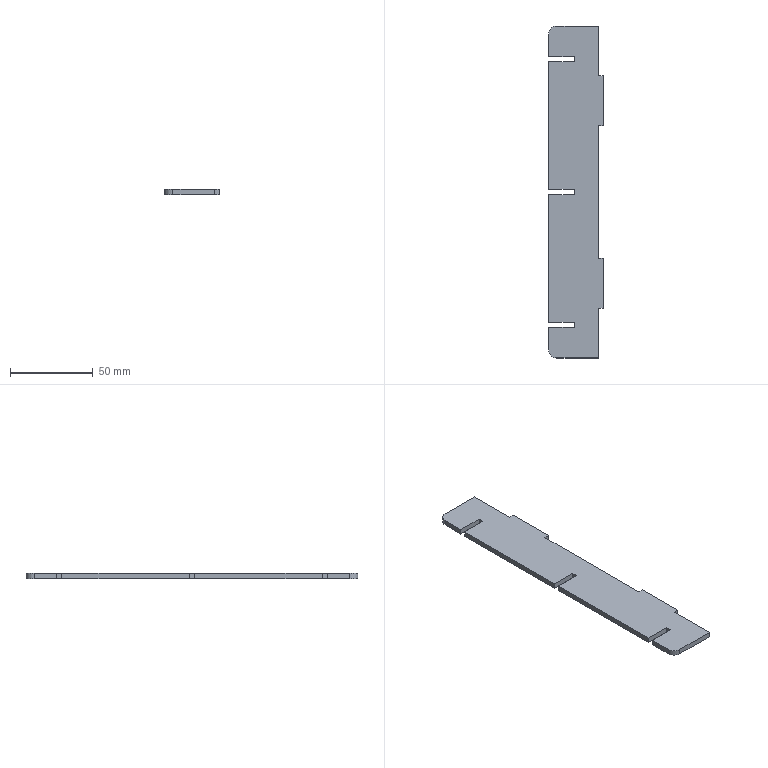Part | SolidWorks | features FlatPattern 1, SMBaseFlange 1, SheetMetal 1 | 1 solid | 28 faces | box 33 x 200 x 3.2 mm | volume 19266 mm3 | plane 26 | cylinder 2 | commonest cylinder face diameters 10 x2
STEP:
#1=CARTESIAN_POINT('',(108.501,81.943,0.));
#2=VERTEX_POINT('',#1);
#3=CARTESIAN_POINT('',(108.501,111.943,0.));
#4=VERTEX_POINT('',#3);
#5=CARTESIAN_POINT('',(108.501,111.943,0.));
#6=DIRECTION('',(0.,1.,0.));
#7=VECTOR('',#6,1000.);
#8=LINE('',#5,#7);
#9=EDGE_CURVE('',#2,#4,#8,.T.);
#10=ORIENTED_EDGE('',*,*,#9,.F.);
#11=CARTESIAN_POINT('',(108.501,81.943,-3.2));
#12=VERTEX_POINT('',#11);
#13=CARTESIAN_POINT('',(108.501,81.943,-3.2));
#14=DIRECTION('',(0.,0.,1.));
#15=VECTOR('',#14,1000.);
#16=LINE('',#13,#15);
#17=EDGE_CURVE('',#12,#2,#16,.T.);
#18=ORIENTED_EDGE('',*,*,#17,.F.);
#19=CARTESIAN_POINT('',(108.501,111.943,-3.2));
#20=VERTEX_POINT('',#19);
#21=CARTESIAN_POINT('',(108.501,111.943,-3.2));
#22=DIRECTION('',(0.,1.,0.));
#23=VECTOR('',#22,1000.);
#24=LINE('',#21,#23);
#25=EDGE_CURVE('',#12,#20,#24,.T.);
#26=ORIENTED_EDGE('',*,*,#25,.T.);
#27=CARTESIAN_POINT('',(108.501,111.943,-3.2));
#28=DIRECTION('',(0.,0.,1.));
#29=VECTOR('',#28,1000.);
#30=LINE('',#27,#29);
#31=EDGE_CURVE('',#20,#4,#30,.T.);
#32=ORIENTED_EDGE('',*,*,#31,.T.);
#33=EDGE_LOOP('',(#10,#18,#26,#32));
#34=FACE_OUTER_BOUND('',#33,.T.);
#35=CARTESIAN_POINT('',(108.501,111.943,-3.2));
#36=DIRECTION('',(1.,0.,0.));
#37=DIRECTION('',(0.,0.,-1.));
#38=AXIS2_PLACEMENT_3D('',#35,#36,#37);
#39=PLANE('',#38);
#40=ADVANCED_FACE('',(#34),#39,.T.);
#41=CARTESIAN_POINT('',(111.501,81.943,0.));
#42=VERTEX_POINT('',#41);
#43=CARTESIAN_POINT('',(108.501,81.943,0.));
#44=DIRECTION('',(-1.,0.,0.));
#45=VECTOR('',#44,1000.);
#46=LINE('',#43,#45);
#47=EDGE_CURVE('',#42,#2,#46,.T.);
#48=ORIENTED_EDGE('',*,*,#47,.F.);
#49=CARTESIAN_POINT('',(111.501,81.943,-3.2));
#50=VERTEX_POINT('',#49);
#51=CARTESIAN_POINT('',(111.501,81.943,-3.2));
#52=DIRECTION('',(0.,0.,1.));
#53=VECTOR('',#52,1000.);
#54=LINE('',#51,#53);
#55=EDGE_CURVE('',#50,#42,#54,.T.);
#56=ORIENTED_EDGE('',*,*,#55,.F.);
#57=CARTESIAN_POINT('',(108.501,81.943,-3.2));
#58=DIRECTION('',(-1.,0.,0.));
#59=VECTOR('',#58,1000.);
#60=LINE('',#57,#59);
#61=EDGE_CURVE('',#50,#12,#60,.T.);
#62=ORIENTED_EDGE('',*,*,#61,.T.);
#63=ORIENTED_EDGE('',*,*,#17,.T.);
#64=EDGE_LOOP('',(#48,#56,#62,#63));
#65=FACE_OUTER_BOUND('',#64,.T.);
#66=CARTESIAN_POINT('',(108.501,81.943,-3.2));
#67=DIRECTION('',(0.,1.,0.));
#68=DIRECTION('',(0.,0.,1.));
#69=AXIS2_PLACEMENT_3D('',#66,#67,#68);
#70=PLANE('',#69);
#71=ADVANCED_FACE('',(#65),#70,.T.);
#72=CARTESIAN_POINT('',(111.501,51.943,0.));
#73=VERTEX_POINT('',#72);
#74=CARTESIAN_POINT('',(111.501,81.943,0.));
#75=DIRECTION('',(0.,1.,0.));
#76=VECTOR('',#75,1000.);
#77=LINE('',#74,#76);
#78=EDGE_CURVE('',#73,#42,#77,.T.);
#79=ORIENTED_EDGE('',*,*,#78,.F.);
#80=CARTESIAN_POINT('',(111.501,51.943,-3.2));
#81=VERTEX_POINT('',#80);
#82=CARTESIAN_POINT('',(111.501,51.943,-3.2));
#83=DIRECTION('',(0.,0.,1.));
#84=VECTOR('',#83,1000.);
#85=LINE('',#82,#84);
#86=EDGE_CURVE('',#81,#73,#85,.T.);
#87=ORIENTED_EDGE('',*,*,#86,.F.);
#88=CARTESIAN_POINT('',(111.501,81.943,-3.2));
#89=DIRECTION('',(0.,1.,0.));
#90=VECTOR('',#89,1000.);
#91=LINE('',#88,#90);
#92=EDGE_CURVE('',#81,#50,#91,.T.);
#93=ORIENTED_EDGE('',*,*,#92,.T.);
#94=ORIENTED_EDGE('',*,*,#55,.T.);
#95=EDGE_LOOP('',(#79,#87,#93,#94));
#96=FACE_OUTER_BOUND('',#95,.T.);
#97=CARTESIAN_POINT('',(111.501,81.943,-3.2));
#98=DIRECTION('',(1.,0.,0.));
#99=DIRECTION('',(0.,1.,0.));
#100=AXIS2_PLACEMENT_3D('',#97,#98,#99);
#101=PLANE('',#100);
#102=ADVANCED_FACE('',(#96),#101,.T.);
#103=CARTESIAN_POINT('',(108.501,51.943,0.));
#104=VERTEX_POINT('',#103);
#105=CARTESIAN_POINT('',(111.501,51.943,0.));
#106=DIRECTION('',(1.,0.,0.));
#107=VECTOR('',#106,1000.);
#108=LINE('',#105,#107);
#109=EDGE_CURVE('',#104,#73,#108,.T.);
#110=ORIENTED_EDGE('',*,*,#109,.F.);
#111=CARTESIAN_POINT('',(108.501,51.943,-3.2));
#112=VERTEX_POINT('',#111);
#113=CARTESIAN_POINT('',(108.501,51.943,-3.2));
#114=DIRECTION('',(0.,0.,1.));
#115=VECTOR('',#114,1000.);
#116=LINE('',#113,#115);
#117=EDGE_CURVE('',#112,#104,#116,.T.);
#118=ORIENTED_EDGE('',*,*,#117,.F.);
#119=CARTESIAN_POINT('',(111.501,51.943,-3.2));
#120=DIRECTION('',(1.,0.,0.));
#121=VECTOR('',#120,1000.);
#122=LINE('',#119,#121);
#123=EDGE_CURVE('',#112,#81,#122,.T.);
#124=ORIENTED_EDGE('',*,*,#123,.T.);
#125=ORIENTED_EDGE('',*,*,#86,.T.);
#126=EDGE_LOOP('',(#110,#118,#124,#125));
#127=FACE_OUTER_BOUND('',#126,.T.);
#128=CARTESIAN_POINT('',(111.501,51.943,-3.2));
#129=DIRECTION('',(0.,-1.,0.));
#130=DIRECTION('',(0.,0.,-1.));
#131=AXIS2_PLACEMENT_3D('',#128,#129,#130);
#132=PLANE('',#131);
#133=ADVANCED_FACE('',(#127),#132,.T.);
#134=CARTESIAN_POINT('',(108.501,-28.057,0.));
#135=VERTEX_POINT('',#134);
#136=CARTESIAN_POINT('',(108.501,51.943,0.));
#137=DIRECTION('',(0.,1.,0.));
#138=VECTOR('',#137,1000.);
#139=LINE('',#136,#138);
#140=EDGE_CURVE('',#135,#104,#139,.T.);
#141=ORIENTED_EDGE('',*,*,#140,.F.);
#142=CARTESIAN_POINT('',(108.501,-28.057,-3.2));
#143=VERTEX_POINT('',#142);
#144=CARTESIAN_POINT('',(108.501,-28.057,-3.2));
#145=DIRECTION('',(0.,0.,1.));
#146=VECTOR('',#145,1000.);
#147=LINE('',#144,#146);
#148=EDGE_CURVE('',#143,#135,#147,.T.);
#149=ORIENTED_EDGE('',*,*,#148,.F.);
#150=CARTESIAN_POINT('',(108.501,51.943,-3.2));
#151=DIRECTION('',(0.,1.,0.));
#152=VECTOR('',#151,1000.);
#153=LINE('',#150,#152);
#154=EDGE_CURVE('',#143,#112,#153,.T.);
#155=ORIENTED_EDGE('',*,*,#154,.T.);
#156=ORIENTED_EDGE('',*,*,#117,.T.);
#157=EDGE_LOOP('',(#141,#149,#155,#156));
#158=FACE_OUTER_BOUND('',#157,.T.);
#159=CARTESIAN_POINT('',(108.501,51.943,-3.2));
#160=DIRECTION('',(1.,0.,0.));
#161=DIRECTION('',(0.,0.,-1.));
#162=AXIS2_PLACEMENT_3D('',#159,#160,#161);
#163=PLANE('',#162);
#164=ADVANCED_FACE('',(#158),#163,.T.);
#165=CARTESIAN_POINT('',(111.501,-28.057,0.));
#166=VERTEX_POINT('',#165);
#167=CARTESIAN_POINT('',(111.501,-28.057,0.));
#168=DIRECTION('',(-1.,0.,0.));
#169=VECTOR('',#168,1000.);
#170=LINE('',#167,#169);
#171=EDGE_CURVE('',#166,#135,#170,.T.);
#172=ORIENTED_EDGE('',*,*,#171,.F.);
#173=CARTESIAN_POINT('',(111.501,-28.057,-3.2));
#174=VERTEX_POINT('',#173);
#175=CARTESIAN_POINT('',(111.501,-28.057,-3.2));
#176=DIRECTION('',(0.,0.,1.));
#177=VECTOR('',#176,1000.);
#178=LINE('',#175,#177);
#179=EDGE_CURVE('',#174,#166,#178,.T.);
#180=ORIENTED_EDGE('',*,*,#179,.F.);
#181=CARTESIAN_POINT('',(111.501,-28.057,-3.2));
#182=DIRECTION('',(-1.,0.,0.));
#183=VECTOR('',#182,1000.);
#184=LINE('',#181,#183);
#185=EDGE_CURVE('',#174,#143,#184,.T.);
#186=ORIENTED_EDGE('',*,*,#185,.T.);
#187=ORIENTED_EDGE('',*,*,#148,.T.);
#188=EDGE_LOOP('',(#172,#180,#186,#187));
#189=FACE_OUTER_BOUND('',#188,.T.);
#190=CARTESIAN_POINT('',(111.501,-28.057,-3.2));
#191=DIRECTION('',(0.,1.,0.));
#192=DIRECTION('',(0.,0.,1.));
#193=AXIS2_PLACEMENT_3D('',#190,#191,#192);
#194=PLANE('',#193);
#195=ADVANCED_FACE('',(#189),#194,.T.);
#196=CARTESIAN_POINT('',(111.501,-58.057,0.));
#197=VERTEX_POINT('',#196);
#198=CARTESIAN_POINT('',(111.501,-58.057,0.));
#199=DIRECTION('',(0.,1.,0.));
#200=VECTOR('',#199,1000.);
#201=LINE('',#198,#200);
#202=EDGE_CURVE('',#197,#166,#201,.T.);
#203=ORIENTED_EDGE('',*,*,#202,.F.);
#204=CARTESIAN_POINT('',(111.501,-58.057,-3.2));
#205=VERTEX_POINT('',#204);
#206=CARTESIAN_POINT('',(111.501,-58.057,-3.2));
#207=DIRECTION('',(0.,0.,1.));
#208=VECTOR('',#207,1000.);
#209=LINE('',#206,#208);
#210=EDGE_CURVE('',#205,#197,#209,.T.);
#211=ORIENTED_EDGE('',*,*,#210,.F.);
#212=CARTESIAN_POINT('',(111.501,-58.057,-3.2));
#213=DIRECTION('',(0.,1.,0.));
#214=VECTOR('',#213,1000.);
#215=LINE('',#212,#214);
#216=EDGE_CURVE('',#205,#174,#215,.T.);
#217=ORIENTED_EDGE('',*,*,#216,.T.);
#218=ORIENTED_EDGE('',*,*,#179,.T.);
#219=EDGE_LOOP('',(#203,#211,#217,#218));
#220=FACE_OUTER_BOUND('',#219,.T.);
#221=CARTESIAN_POINT('',(111.501,-58.057,-3.2));
#222=DIRECTION('',(1.,0.,0.));
#223=DIRECTION('',(0.,0.,-1.));
#224=AXIS2_PLACEMENT_3D('',#221,#222,#223);
#225=PLANE('',#224);
#226=ADVANCED_FACE('',(#220),#225,.T.);
#227=CARTESIAN_POINT('',(108.501,-58.057,0.));
#228=VERTEX_POINT('',#227);
#229=CARTESIAN_POINT('',(108.501,-58.057,0.));
#230=DIRECTION('',(1.,0.,0.));
#231=VECTOR('',#230,1000.);
#232=LINE('',#229,#231);
#233=EDGE_CURVE('',#228,#197,#232,.T.);
#234=ORIENTED_EDGE('',*,*,#233,.F.);
#235=CARTESIAN_POINT('',(108.501,-58.057,-3.2));
#236=VERTEX_POINT('',#235);
#237=CARTESIAN_POINT('',(108.501,-58.057,-3.2));
#238=DIRECTION('',(0.,0.,1.));
#239=VECTOR('',#238,1000.);
#240=LINE('',#237,#239);
#241=EDGE_CURVE('',#236,#228,#240,.T.);
#242=ORIENTED_EDGE('',*,*,#241,.F.);
#243=CARTESIAN_POINT('',(108.501,-58.057,-3.2));
#244=DIRECTION('',(1.,0.,0.));
#245=VECTOR('',#244,1000.);
#246=LINE('',#243,#245);
#247=EDGE_CURVE('',#236,#205,#246,.T.);
#248=ORIENTED_EDGE('',*,*,#247,.T.);
#249=ORIENTED_EDGE('',*,*,#210,.T.);
#250=EDGE_LOOP('',(#234,#242,#248,#249));
#251=FACE_OUTER_BOUND('',#250,.T.);
#252=CARTESIAN_POINT('',(108.501,-58.057,-3.2));
#253=DIRECTION('',(0.,-1.,0.));
#254=DIRECTION('',(0.,0.,-1.));
#255=AXIS2_PLACEMENT_3D('',#252,#253,#254);
#256=PLANE('',#255);
#257=ADVANCED_FACE('',(#251),#256,.T.);
#258=CARTESIAN_POINT('',(108.501,-88.057,0.));
#259=VERTEX_POINT('',#258);
#260=CARTESIAN_POINT('',(108.501,-58.057,0.));
#261=DIRECTION('',(0.,1.,0.));
#262=VECTOR('',#261,1000.);
#263=LINE('',#260,#262);
#264=EDGE_CURVE('',#259,#228,#263,.T.);
#265=ORIENTED_EDGE('',*,*,#264,.F.);
#266=CARTESIAN_POINT('',(108.501,-88.057,-3.2));
#267=VERTEX_POINT('',#266);
#268=CARTESIAN_POINT('',(108.501,-88.057,-3.2));
#269=DIRECTION('',(0.,0.,1.));
#270=VECTOR('',#269,1000.);
#271=LINE('',#268,#270);
#272=EDGE_CURVE('',#267,#259,#271,.T.);
#273=ORIENTED_EDGE('',*,*,#272,.F.);
#274=CARTESIAN_POINT('',(108.501,-58.057,-3.2));
#275=DIRECTION('',(0.,1.,0.));
#276=VECTOR('',#275,1000.);
#277=LINE('',#274,#276);
#278=EDGE_CURVE('',#267,#236,#277,.T.);
#279=ORIENTED_EDGE('',*,*,#278,.T.);
#280=ORIENTED_EDGE('',*,*,#241,.T.);
#281=EDGE_LOOP('',(#265,#273,#279,#280));
#282=FACE_OUTER_BOUND('',#281,.T.);
#283=CARTESIAN_POINT('',(108.501,-58.057,-3.2));
#284=DIRECTION('',(1.,0.,0.));
#285=DIRECTION('',(0.,1.,0.));
#286=AXIS2_PLACEMENT_3D('',#283,#284,#285);
#287=PLANE('',#286);
#288=ADVANCED_FACE('',(#282),#287,.T.);
#289=CARTESIAN_POINT('',(83.501,-88.057,0.));
#290=VERTEX_POINT('',#289);
#291=CARTESIAN_POINT('',(108.501,-88.057,0.));
#292=DIRECTION('',(1.,0.,0.));
#293=VECTOR('',#292,1000.);
#294=LINE('',#291,#293);
#295=EDGE_CURVE('',#290,#259,#294,.T.);
#296=ORIENTED_EDGE('',*,*,#295,.F.);
#297=CARTESIAN_POINT('',(83.501,-88.057,-3.2));
#298=VERTEX_POINT('',#297);
#299=CARTESIAN_POINT('',(83.501,-88.057,-3.2));
#300=DIRECTION('',(0.,0.,1.));
#301=VECTOR('',#300,1000.);
#302=LINE('',#299,#301);
#303=EDGE_CURVE('',#298,#290,#302,.T.);
#304=ORIENTED_EDGE('',*,*,#303,.F.);
#305=CARTESIAN_POINT('',(108.501,-88.057,-3.2));
#306=DIRECTION('',(1.,0.,0.));
#307=VECTOR('',#306,1000.);
#308=LINE('',#305,#307);
#309=EDGE_CURVE('',#298,#267,#308,.T.);
#310=ORIENTED_EDGE('',*,*,#309,.T.);
#311=ORIENTED_EDGE('',*,*,#272,.T.);
#312=EDGE_LOOP('',(#296,#304,#310,#311));
#313=FACE_OUTER_BOUND('',#312,.T.);
#314=CARTESIAN_POINT('',(108.501,-88.057,-3.2));
#315=DIRECTION('',(0.,-1.,0.));
#316=DIRECTION('',(0.,0.,-1.));
#317=AXIS2_PLACEMENT_3D('',#314,#315,#316);
#318=PLANE('',#317);
#319=ADVANCED_FACE('',(#313),#318,.T.);
#320=CARTESIAN_POINT('',(78.501,-83.057,0.));
#321=VERTEX_POINT('',#320);
#322=CARTESIAN_POINT('',(83.501,-83.057,0.));
#323=DIRECTION('',(0.,0.,1.));
#324=DIRECTION('',(-1.,0.,0.));
#325=AXIS2_PLACEMENT_3D('',#322,#323,#324);
#326=CIRCLE('',#325,5.);
#327=EDGE_CURVE('',#321,#290,#326,.T.);
#328=ORIENTED_EDGE('',*,*,#327,.F.);
#329=CARTESIAN_POINT('',(78.501,-83.057,-3.2));
#330=VERTEX_POINT('',#329);
#331=CARTESIAN_POINT('',(78.501,-83.057,-3.2));
#332=DIRECTION('',(0.,0.,1.));
#333=VECTOR('',#332,1000.);
#334=LINE('',#331,#333);
#335=EDGE_CURVE('',#330,#321,#334,.T.);
#336=ORIENTED_EDGE('',*,*,#335,.F.);
#337=CARTESIAN_POINT('',(83.501,-83.057,-3.2));
#338=DIRECTION('',(0.,0.,1.));
#339=DIRECTION('',(-1.,0.,0.));
#340=AXIS2_PLACEMENT_3D('',#337,#338,#339);
#341=CIRCLE('',#340,5.);
#342=EDGE_CURVE('',#330,#298,#341,.T.);
#343=ORIENTED_EDGE('',*,*,#342,.T.);
#344=ORIENTED_EDGE('',*,*,#303,.T.);
#345=EDGE_LOOP('',(#328,#336,#343,#344));
#346=FACE_OUTER_BOUND('',#345,.T.);
#347=CARTESIAN_POINT('',(83.501,-83.057,-3.2));
#348=DIRECTION('',(0.,0.,1.));
#349=DIRECTION('',(1.,0.,0.));
#350=AXIS2_PLACEMENT_3D('',#347,#348,#349);
#351=CYLINDRICAL_SURFACE('',#350,5.);
#352=ADVANCED_FACE('',(#346),#351,.T.);
#353=CARTESIAN_POINT('',(78.501,-69.657,0.));
#354=VERTEX_POINT('',#353);
#355=CARTESIAN_POINT('',(78.501,-69.657,0.));
#356=DIRECTION('',(0.,-1.,0.));
#357=VECTOR('',#356,1000.);
#358=LINE('',#355,#357);
#359=EDGE_CURVE('',#354,#321,#358,.T.);
#360=ORIENTED_EDGE('',*,*,#359,.F.);
#361=CARTESIAN_POINT('',(78.501,-69.657,-3.2));
#362=VERTEX_POINT('',#361);
#363=CARTESIAN_POINT('',(78.501,-69.657,-3.2));
#364=DIRECTION('',(0.,0.,1.));
#365=VECTOR('',#364,1000.);
#366=LINE('',#363,#365);
#367=EDGE_CURVE('',#362,#354,#366,.T.);
#368=ORIENTED_EDGE('',*,*,#367,.F.);
#369=CARTESIAN_POINT('',(78.501,-69.657,-3.2));
#370=DIRECTION('',(0.,-1.,0.));
#371=VECTOR('',#370,1000.);
#372=LINE('',#369,#371);
#373=EDGE_CURVE('',#362,#330,#372,.T.);
#374=ORIENTED_EDGE('',*,*,#373,.T.);
#375=ORIENTED_EDGE('',*,*,#335,.T.);
#376=EDGE_LOOP('',(#360,#368,#374,#375));
#377=FACE_OUTER_BOUND('',#376,.T.);
#378=CARTESIAN_POINT('',(78.501,-69.657,-3.2));
#379=DIRECTION('',(-1.,0.,0.));
#380=DIRECTION('',(0.,0.,1.));
#381=AXIS2_PLACEMENT_3D('',#378,#379,#380);
#382=PLANE('',#381);
#383=ADVANCED_FACE('',(#377),#382,.T.);
#384=CARTESIAN_POINT('',(94.001,-69.657,0.));
#385=VERTEX_POINT('',#384);
#386=CARTESIAN_POINT('',(94.001,-69.657,0.));
#387=DIRECTION('',(-1.,0.,0.));
#388=VECTOR('',#387,1000.);
#389=LINE('',#386,#388);
#390=EDGE_CURVE('',#385,#354,#389,.T.);
#391=ORIENTED_EDGE('',*,*,#390,.F.);
#392=CARTESIAN_POINT('',(94.001,-69.657,-3.2));
#393=VERTEX_POINT('',#392);
#394=CARTESIAN_POINT('',(94.001,-69.657,-3.2));
#395=DIRECTION('',(0.,0.,1.));
#396=VECTOR('',#395,1000.);
#397=LINE('',#394,#396);
#398=EDGE_CURVE('',#393,#385,#397,.T.);
#399=ORIENTED_EDGE('',*,*,#398,.F.);
#400=CARTESIAN_POINT('',(94.001,-69.657,-3.2));
#401=DIRECTION('',(-1.,0.,0.));
#402=VECTOR('',#401,1000.);
#403=LINE('',#400,#402);
#404=EDGE_CURVE('',#393,#362,#403,.T.);
#405=ORIENTED_EDGE('',*,*,#404,.T.);
#406=ORIENTED_EDGE('',*,*,#367,.T.);
#407=EDGE_LOOP('',(#391,#399,#405,#406));
#408=FACE_OUTER_BOUND('',#407,.T.);
#409=CARTESIAN_POINT('',(94.001,-69.657,-3.2));
#410=DIRECTION('',(0.,1.,0.));
#411=DIRECTION('',(0.,0.,1.));
#412=AXIS2_PLACEMENT_3D('',#409,#410,#411);
#413=PLANE('',#412);
#414=ADVANCED_FACE('',(#408),#413,.T.);
#415=CARTESIAN_POINT('',(94.001,-66.457,0.));
#416=VERTEX_POINT('',#415);
#417=CARTESIAN_POINT('',(94.001,-66.457,0.));
#418=DIRECTION('',(0.,-1.,0.));
#419=VECTOR('',#418,1000.);
#420=LINE('',#417,#419);
#421=EDGE_CURVE('',#416,#385,#420,.T.);
#422=ORIENTED_EDGE('',*,*,#421,.F.);
#423=CARTESIAN_POINT('',(94.001,-66.457,-3.2));
#424=VERTEX_POINT('',#423);
#425=CARTESIAN_POINT('',(94.001,-66.457,-3.2));
#426=DIRECTION('',(0.,0.,1.));
#427=VECTOR('',#426,1000.);
#428=LINE('',#425,#427);
#429=EDGE_CURVE('',#424,#416,#428,.T.);
#430=ORIENTED_EDGE('',*,*,#429,.F.);
#431=CARTESIAN_POINT('',(94.001,-66.457,-3.2));
#432=DIRECTION('',(0.,-1.,0.));
#433=VECTOR('',#432,1000.);
#434=LINE('',#431,#433);
#435=EDGE_CURVE('',#424,#393,#434,.T.);
#436=ORIENTED_EDGE('',*,*,#435,.T.);
#437=ORIENTED_EDGE('',*,*,#398,.T.);
#438=EDGE_LOOP('',(#422,#430,#436,#437));
#439=FACE_OUTER_BOUND('',#438,.T.);
#440=CARTESIAN_POINT('',(94.001,-66.457,-3.2));
#441=DIRECTION('',(-1.,0.,0.));
#442=DIRECTION('',(0.,0.,1.));
#443=AXIS2_PLACEMENT_3D('',#440,#441,#442);
#444=PLANE('',#443);
#445=ADVANCED_FACE('',(#439),#444,.T.);
#446=CARTESIAN_POINT('',(78.501,-66.457,0.));
#447=VERTEX_POINT('',#446);
#448=CARTESIAN_POINT('',(78.501,-66.457,0.));
#449=DIRECTION('',(1.,0.,0.));
#450=VECTOR('',#449,1000.);
#451=LINE('',#448,#450);
#452=EDGE_CURVE('',#447,#416,#451,.T.);
#453=ORIENTED_EDGE('',*,*,#452,.F.);
#454=CARTESIAN_POINT('',(78.501,-66.457,-3.2));
#455=VERTEX_POINT('',#454);
#456=CARTESIAN_POINT('',(78.501,-66.457,-3.2));
#457=DIRECTION('',(0.,0.,1.));
#458=VECTOR('',#457,1000.);
#459=LINE('',#456,#458);
#460=EDGE_CURVE('',#455,#447,#459,.T.);
#461=ORIENTED_EDGE('',*,*,#460,.F.);
#462=CARTESIAN_POINT('',(78.501,-66.457,-3.2));
#463=DIRECTION('',(1.,0.,0.));
#464=VECTOR('',#463,1000.);
#465=LINE('',#462,#464);
#466=EDGE_CURVE('',#455,#424,#465,.T.);
#467=ORIENTED_EDGE('',*,*,#466,.T.);
#468=ORIENTED_EDGE('',*,*,#429,.T.);
#469=EDGE_LOOP('',(#453,#461,#467,#468));
#470=FACE_OUTER_BOUND('',#469,.T.);
#471=CARTESIAN_POINT('',(78.501,-66.457,-3.2));
#472=DIRECTION('',(0.,-1.,0.));
#473=DIRECTION('',(0.,0.,-1.));
#474=AXIS2_PLACEMENT_3D('',#471,#472,#473);
#475=PLANE('',#474);
#476=ADVANCED_FACE('',(#470),#475,.T.);
#477=CARTESIAN_POINT('',(78.501,10.343,0.));
#478=VERTEX_POINT('',#477);
#479=CARTESIAN_POINT('',(78.501,10.343,0.));
#480=DIRECTION('',(0.,-1.,0.));
#481=VECTOR('',#480,1000.);
#482=LINE('',#479,#481);
#483=EDGE_CURVE('',#478,#447,#482,.T.);
#484=ORIENTED_EDGE('',*,*,#483,.F.);
#485=CARTESIAN_POINT('',(78.501,10.343,-3.2));
#486=VERTEX_POINT('',#485);
#487=CARTESIAN_POINT('',(78.501,10.343,-3.2));
#488=DIRECTION('',(0.,0.,1.));
#489=VECTOR('',#488,1000.);
#490=LINE('',#487,#489);
#491=EDGE_CURVE('',#486,#478,#490,.T.);
#492=ORIENTED_EDGE('',*,*,#491,.F.);
#493=CARTESIAN_POINT('',(78.501,10.343,-3.2));
#494=DIRECTION('',(0.,-1.,0.));
#495=VECTOR('',#494,1000.);
#496=LINE('',#493,#495);
#497=EDGE_CURVE('',#486,#455,#496,.T.);
#498=ORIENTED_EDGE('',*,*,#497,.T.);
#499=ORIENTED_EDGE('',*,*,#460,.T.);
#500=EDGE_LOOP('',(#484,#492,#498,#499));
#501=FACE_OUTER_BOUND('',#500,.T.);
#502=CARTESIAN_POINT('',(78.501,10.343,-3.2));
#503=DIRECTION('',(-1.,0.,0.));
#504=DIRECTION('',(0.,0.,1.));
#505=AXIS2_PLACEMENT_3D('',#502,#503,#504);
#506=PLANE('',#505);
#507=ADVANCED_FACE('',(#501),#506,.T.);
#508=CARTESIAN_POINT('',(94.001,10.343,0.));
#509=VERTEX_POINT('',#508);
#510=CARTESIAN_POINT('',(94.001,10.343,0.));
#511=DIRECTION('',(-1.,0.,0.));
#512=VECTOR('',#511,1000.);
#513=LINE('',#510,#512);
#514=EDGE_CURVE('',#509,#478,#513,.T.);
#515=ORIENTED_EDGE('',*,*,#514,.F.);
#516=CARTESIAN_POINT('',(94.001,10.343,-3.2));
#517=VERTEX_POINT('',#516);
#518=CARTESIAN_POINT('',(94.001,10.343,-3.2));
#519=DIRECTION('',(0.,0.,1.));
#520=VECTOR('',#519,1000.);
#521=LINE('',#518,#520);
#522=EDGE_CURVE('',#517,#509,#521,.T.);
#523=ORIENTED_EDGE('',*,*,#522,.F.);
#524=CARTESIAN_POINT('',(94.001,10.343,-3.2));
#525=DIRECTION('',(-1.,0.,0.));
#526=VECTOR('',#525,1000.);
#527=LINE('',#524,#526);
#528=EDGE_CURVE('',#517,#486,#527,.T.);
#529=ORIENTED_EDGE('',*,*,#528,.T.);
#530=ORIENTED_EDGE('',*,*,#491,.T.);
#531=EDGE_LOOP('',(#515,#523,#529,#530));
#532=FACE_OUTER_BOUND('',#531,.T.);
#533=CARTESIAN_POINT('',(94.001,10.343,-3.2));
#534=DIRECTION('',(0.,1.,0.));
#535=DIRECTION('',(-1.,0.,0.));
#536=AXIS2_PLACEMENT_3D('',#533,#534,#535);
#537=PLANE('',#536);
#538=ADVANCED_FACE('',(#532),#537,.T.);
#539=CARTESIAN_POINT('',(94.001,13.543,0.));
#540=VERTEX_POINT('',#539);
#541=CARTESIAN_POINT('',(94.001,13.543,0.));
#542=DIRECTION('',(0.,-1.,0.));
#543=VECTOR('',#542,1000.);
#544=LINE('',#541,#543);
#545=EDGE_CURVE('',#540,#509,#544,.T.);
#546=ORIENTED_EDGE('',*,*,#545,.F.);
#547=CARTESIAN_POINT('',(94.001,13.543,-3.2));
#548=VERTEX_POINT('',#547);
#549=CARTESIAN_POINT('',(94.001,13.543,-3.2));
#550=DIRECTION('',(0.,0.,1.));
#551=VECTOR('',#550,1000.);
#552=LINE('',#549,#551);
#553=EDGE_CURVE('',#548,#540,#552,.T.);
#554=ORIENTED_EDGE('',*,*,#553,.F.);
#555=CARTESIAN_POINT('',(94.001,13.543,-3.2));
#556=DIRECTION('',(0.,-1.,0.));
#557=VECTOR('',#556,1000.);
#558=LINE('',#555,#557);
#559=EDGE_CURVE('',#548,#517,#558,.T.);
#560=ORIENTED_EDGE('',*,*,#559,.T.);
#561=ORIENTED_EDGE('',*,*,#522,.T.);
#562=EDGE_LOOP('',(#546,#554,#560,#561));
#563=FACE_OUTER_BOUND('',#562,.T.);
#564=CARTESIAN_POINT('',(94.001,13.543,-3.2));
#565=DIRECTION('',(-1.,0.,0.));
#566=DIRECTION('',(0.,-1.,0.));
#567=AXIS2_PLACEMENT_3D('',#564,#565,#566);
#568=PLANE('',#567);
#569=ADVANCED_FACE('',(#563),#568,.T.);
#570=CARTESIAN_POINT('',(78.501,13.543,0.));
#571=VERTEX_POINT('',#570);
#572=CARTESIAN_POINT('',(78.501,13.543,0.));
#573=DIRECTION('',(1.,0.,0.));
#574=VECTOR('',#573,1000.);
#575=LINE('',#572,#574);
#576=EDGE_CURVE('',#571,#540,#575,.T.);
#577=ORIENTED_EDGE('',*,*,#576,.F.);
#578=CARTESIAN_POINT('',(78.501,13.543,-3.2));
#579=VERTEX_POINT('',#578);
#580=CARTESIAN_POINT('',(78.501,13.543,-3.2));
#581=DIRECTION('',(0.,0.,1.));
#582=VECTOR('',#581,1000.);
#583=LINE('',#580,#582);
#584=EDGE_CURVE('',#579,#571,#583,.T.);
#585=ORIENTED_EDGE('',*,*,#584,.F.);
#586=CARTESIAN_POINT('',(78.501,13.543,-3.2));
#587=DIRECTION('',(1.,0.,0.));
#588=VECTOR('',#587,1000.);
#589=LINE('',#586,#588);
#590=EDGE_CURVE('',#579,#548,#589,.T.);
#591=ORIENTED_EDGE('',*,*,#590,.T.);
#592=ORIENTED_EDGE('',*,*,#553,.T.);
#593=EDGE_LOOP('',(#577,#585,#591,#592));
#594=FACE_OUTER_BOUND('',#593,.T.);
#595=CARTESIAN_POINT('',(78.501,13.543,-3.2));
#596=DIRECTION('',(0.,-1.,0.));
#597=DIRECTION('',(1.,0.,0.));
#598=AXIS2_PLACEMENT_3D('',#595,#596,#597);
#599=PLANE('',#598);
#600=ADVANCED_FACE('',(#594),#599,.T.);
#601=CARTESIAN_POINT('',(78.501,90.343,0.));
#602=VERTEX_POINT('',#601);
#603=CARTESIAN_POINT('',(78.501,90.343,0.));
#604=DIRECTION('',(0.,-1.,0.));
#605=VECTOR('',#604,1000.);
#606=LINE('',#603,#605);
#607=EDGE_CURVE('',#602,#571,#606,.T.);
#608=ORIENTED_EDGE('',*,*,#607,.F.);
#609=CARTESIAN_POINT('',(78.501,90.343,-3.2));
#610=VERTEX_POINT('',#609);
#611=CARTESIAN_POINT('',(78.501,90.343,-3.2));
#612=DIRECTION('',(0.,0.,1.));
#613=VECTOR('',#612,1000.);
#614=LINE('',#611,#613);
#615=EDGE_CURVE('',#610,#602,#614,.T.);
#616=ORIENTED_EDGE('',*,*,#615,.F.);
#617=CARTESIAN_POINT('',(78.501,90.343,-3.2));
#618=DIRECTION('',(0.,-1.,0.));
#619=VECTOR('',#618,1000.);
#620=LINE('',#617,#619);
#621=EDGE_CURVE('',#610,#579,#620,.T.);
#622=ORIENTED_EDGE('',*,*,#621,.T.);
#623=ORIENTED_EDGE('',*,*,#584,.T.);
#624=EDGE_LOOP('',(#608,#616,#622,#623));
#625=FACE_OUTER_BOUND('',#624,.T.);
#626=CARTESIAN_POINT('',(78.501,90.343,-3.2));
#627=DIRECTION('',(-1.,0.,0.));
#628=DIRECTION('',(0.,-1.,0.));
#629=AXIS2_PLACEMENT_3D('',#626,#627,#628);
#630=PLANE('',#629);
#631=ADVANCED_FACE('',(#625),#630,.T.);
#632=CARTESIAN_POINT('',(94.001,90.343,0.));
#633=VERTEX_POINT('',#632);
#634=CARTESIAN_POINT('',(94.001,90.343,0.));
#635=DIRECTION('',(-1.,0.,0.));
#636=VECTOR('',#635,1000.);
#637=LINE('',#634,#636);
#638=EDGE_CURVE('',#633,#602,#637,.T.);
#639=ORIENTED_EDGE('',*,*,#638,.F.);
#640=CARTESIAN_POINT('',(94.001,90.343,-3.2));
#641=VERTEX_POINT('',#640);
#642=CARTESIAN_POINT('',(94.001,90.343,-3.2));
#643=DIRECTION('',(0.,0.,1.));
#644=VECTOR('',#643,1000.);
#645=LINE('',#642,#644);
#646=EDGE_CURVE('',#641,#633,#645,.T.);
#647=ORIENTED_EDGE('',*,*,#646,.F.);
#648=CARTESIAN_POINT('',(94.001,90.343,-3.2));
#649=DIRECTION('',(-1.,0.,0.));
#650=VECTOR('',#649,1000.);
#651=LINE('',#648,#650);
#652=EDGE_CURVE('',#641,#610,#651,.T.);
#653=ORIENTED_EDGE('',*,*,#652,.T.);
#654=ORIENTED_EDGE('',*,*,#615,.T.);
#655=EDGE_LOOP('',(#639,#647,#653,#654));
#656=FACE_OUTER_BOUND('',#655,.T.);
#657=CARTESIAN_POINT('',(94.001,90.343,-3.2));
#658=DIRECTION('',(0.,1.,0.));
#659=DIRECTION('',(0.,0.,1.));
#660=AXIS2_PLACEMENT_3D('',#657,#658,#659);
#661=PLANE('',#660);
#662=ADVANCED_FACE('',(#656),#661,.T.);
#663=CARTESIAN_POINT('',(94.001,93.543,0.));
#664=VERTEX_POINT('',#663);
#665=CARTESIAN_POINT('',(94.001,93.543,0.));
#666=DIRECTION('',(0.,-1.,0.));
#667=VECTOR('',#666,1000.);
#668=LINE('',#665,#667);
#669=EDGE_CURVE('',#664,#633,#668,.T.);
#670=ORIENTED_EDGE('',*,*,#669,.F.);
#671=CARTESIAN_POINT('',(94.001,93.543,-3.2));
#672=VERTEX_POINT('',#671);
#673=CARTESIAN_POINT('',(94.001,93.543,-3.2));
#674=DIRECTION('',(0.,0.,1.));
#675=VECTOR('',#674,1000.);
#676=LINE('',#673,#675);
#677=EDGE_CURVE('',#672,#664,#676,.T.);
#678=ORIENTED_EDGE('',*,*,#677,.F.);
#679=CARTESIAN_POINT('',(94.001,93.543,-3.2));
#680=DIRECTION('',(0.,-1.,0.));
#681=VECTOR('',#680,1000.);
#682=LINE('',#679,#681);
#683=EDGE_CURVE('',#672,#641,#682,.T.);
#684=ORIENTED_EDGE('',*,*,#683,.T.);
#685=ORIENTED_EDGE('',*,*,#646,.T.);
#686=EDGE_LOOP('',(#670,#678,#684,#685));
#687=FACE_OUTER_BOUND('',#686,.T.);
#688=CARTESIAN_POINT('',(94.001,93.543,-3.2));
#689=DIRECTION('',(-1.,0.,0.));
#690=DIRECTION('',(0.,0.,1.));
#691=AXIS2_PLACEMENT_3D('',#688,#689,#690);
#692=PLANE('',#691);
#693=ADVANCED_FACE('',(#687),#692,.T.);
#694=CARTESIAN_POINT('',(78.501,93.543,0.));
#695=VERTEX_POINT('',#694);
#696=CARTESIAN_POINT('',(94.001,93.543,0.));
#697=DIRECTION('',(1.,0.,0.));
#698=VECTOR('',#697,1000.);
#699=LINE('',#696,#698);
#700=EDGE_CURVE('',#695,#664,#699,.T.);
#701=ORIENTED_EDGE('',*,*,#700,.F.);
#702=CARTESIAN_POINT('',(78.501,93.543,-3.2));
#703=VERTEX_POINT('',#702);
#704=CARTESIAN_POINT('',(78.501,93.543,-3.2));
#705=DIRECTION('',(0.,0.,1.));
#706=VECTOR('',#705,1000.);
#707=LINE('',#704,#706);
#708=EDGE_CURVE('',#703,#695,#707,.T.);
#709=ORIENTED_EDGE('',*,*,#708,.F.);
#710=CARTESIAN_POINT('',(94.001,93.543,-3.2));
#711=DIRECTION('',(1.,0.,0.));
#712=VECTOR('',#711,1000.);
#713=LINE('',#710,#712);
#714=EDGE_CURVE('',#703,#672,#713,.T.);
#715=ORIENTED_EDGE('',*,*,#714,.T.);
#716=ORIENTED_EDGE('',*,*,#677,.T.);
#717=EDGE_LOOP('',(#701,#709,#715,#716));
#718=FACE_OUTER_BOUND('',#717,.T.);
#719=CARTESIAN_POINT('',(94.001,93.543,-3.2));
#720=DIRECTION('',(0.,-1.,0.));
#721=DIRECTION('',(0.,0.,-1.));
#722=AXIS2_PLACEMENT_3D('',#719,#720,#721);
#723=PLANE('',#722);
#724=ADVANCED_FACE('',(#718),#723,.T.);
#725=CARTESIAN_POINT('',(78.501,106.943,0.));
#726=VERTEX_POINT('',#725);
#727=CARTESIAN_POINT('',(78.501,106.943,0.));
#728=DIRECTION('',(0.,-1.,0.));
#729=VECTOR('',#728,1000.);
#730=LINE('',#727,#729);
#731=EDGE_CURVE('',#726,#695,#730,.T.);
#732=ORIENTED_EDGE('',*,*,#731,.F.);
#733=CARTESIAN_POINT('',(78.501,106.943,-3.2));
#734=VERTEX_POINT('',#733);
#735=CARTESIAN_POINT('',(78.501,106.943,-3.2));
#736=DIRECTION('',(0.,0.,1.));
#737=VECTOR('',#736,1000.);
#738=LINE('',#735,#737);
#739=EDGE_CURVE('',#734,#726,#738,.T.);
#740=ORIENTED_EDGE('',*,*,#739,.F.);
#741=CARTESIAN_POINT('',(78.501,106.943,-3.2));
#742=DIRECTION('',(0.,-1.,0.));
#743=VECTOR('',#742,1000.);
#744=LINE('',#741,#743);
#745=EDGE_CURVE('',#734,#703,#744,.T.);
#746=ORIENTED_EDGE('',*,*,#745,.T.);
#747=ORIENTED_EDGE('',*,*,#708,.T.);
#748=EDGE_LOOP('',(#732,#740,#746,#747));
#749=FACE_OUTER_BOUND('',#748,.T.);
#750=CARTESIAN_POINT('',(78.501,106.943,-3.2));
#751=DIRECTION('',(-1.,0.,0.));
#752=DIRECTION('',(0.,-1.,0.));
#753=AXIS2_PLACEMENT_3D('',#750,#751,#752);
#754=PLANE('',#753);
#755=ADVANCED_FACE('',(#749),#754,.T.);
#756=CARTESIAN_POINT('',(83.501,111.943,0.));
#757=VERTEX_POINT('',#756);
#758=CARTESIAN_POINT('',(83.501,106.943,0.));
#759=DIRECTION('',(0.,0.,1.));
#760=DIRECTION('',(1.,0.,0.));
#761=AXIS2_PLACEMENT_3D('',#758,#759,#760);
#762=CIRCLE('',#761,5.);
#763=EDGE_CURVE('',#757,#726,#762,.T.);
#764=ORIENTED_EDGE('',*,*,#763,.F.);
#765=CARTESIAN_POINT('',(83.501,111.943,-3.2));
#766=VERTEX_POINT('',#765);
#767=CARTESIAN_POINT('',(83.501,111.943,-3.2));
#768=DIRECTION('',(0.,0.,1.));
#769=VECTOR('',#768,1000.);
#770=LINE('',#767,#769);
#771=EDGE_CURVE('',#766,#757,#770,.T.);
#772=ORIENTED_EDGE('',*,*,#771,.F.);
#773=CARTESIAN_POINT('',(83.501,106.943,-3.2));
#774=DIRECTION('',(0.,0.,1.));
#775=DIRECTION('',(1.,0.,0.));
#776=AXIS2_PLACEMENT_3D('',#773,#774,#775);
#777=CIRCLE('',#776,5.);
#778=EDGE_CURVE('',#766,#734,#777,.T.);
#779=ORIENTED_EDGE('',*,*,#778,.T.);
#780=ORIENTED_EDGE('',*,*,#739,.T.);
#781=EDGE_LOOP('',(#764,#772,#779,#780));
#782=FACE_OUTER_BOUND('',#781,.T.);
#783=CARTESIAN_POINT('',(83.501,106.943,-3.2));
#784=DIRECTION('',(0.,0.,1.));
#785=DIRECTION('',(1.,0.,0.));
#786=AXIS2_PLACEMENT_3D('',#783,#784,#785);
#787=CYLINDRICAL_SURFACE('',#786,5.);
#788=ADVANCED_FACE('',(#782),#787,.T.);
#789=CARTESIAN_POINT('',(108.501,111.943,0.));
#790=DIRECTION('',(-1.,0.,0.));
#791=VECTOR('',#790,1000.);
#792=LINE('',#789,#791);
#793=EDGE_CURVE('',#4,#757,#792,.T.);
#794=ORIENTED_EDGE('',*,*,#793,.F.);
#795=ORIENTED_EDGE('',*,*,#31,.F.);
#796=CARTESIAN_POINT('',(108.501,111.943,-3.2));
#797=DIRECTION('',(-1.,0.,0.));
#798=VECTOR('',#797,1000.);
#799=LINE('',#796,#798);
#800=EDGE_CURVE('',#20,#766,#799,.T.);
#801=ORIENTED_EDGE('',*,*,#800,.T.);
#802=ORIENTED_EDGE('',*,*,#771,.T.);
#803=EDGE_LOOP('',(#794,#795,#801,#802));
#804=FACE_OUTER_BOUND('',#803,.T.);
#805=CARTESIAN_POINT('',(108.501,111.943,-3.2));
#806=DIRECTION('',(0.,1.,0.));
#807=DIRECTION('',(0.,0.,1.));
#808=AXIS2_PLACEMENT_3D('',#805,#806,#807);
#809=PLANE('',#808);
#810=ADVANCED_FACE('',(#804),#809,.T.);
#811=ORIENTED_EDGE('',*,*,#25,.F.);
#812=ORIENTED_EDGE('',*,*,#61,.F.);
#813=ORIENTED_EDGE('',*,*,#92,.F.);
#814=ORIENTED_EDGE('',*,*,#123,.F.);
#815=ORIENTED_EDGE('',*,*,#154,.F.);
#816=ORIENTED_EDGE('',*,*,#185,.F.);
#817=ORIENTED_EDGE('',*,*,#216,.F.);
#818=ORIENTED_EDGE('',*,*,#247,.F.);
#819=ORIENTED_EDGE('',*,*,#278,.F.);
#820=ORIENTED_EDGE('',*,*,#309,.F.);
#821=ORIENTED_EDGE('',*,*,#342,.F.);
#822=ORIENTED_EDGE('',*,*,#373,.F.);
#823=ORIENTED_EDGE('',*,*,#404,.F.);
#824=ORIENTED_EDGE('',*,*,#435,.F.);
#825=ORIENTED_EDGE('',*,*,#466,.F.);
#826=ORIENTED_EDGE('',*,*,#497,.F.);
#827=ORIENTED_EDGE('',*,*,#528,.F.);
#828=ORIENTED_EDGE('',*,*,#559,.F.);
#829=ORIENTED_EDGE('',*,*,#590,.F.);
#830=ORIENTED_EDGE('',*,*,#621,.F.);
#831=ORIENTED_EDGE('',*,*,#652,.F.);
#832=ORIENTED_EDGE('',*,*,#683,.F.);
#833=ORIENTED_EDGE('',*,*,#714,.F.);
#834=ORIENTED_EDGE('',*,*,#745,.F.);
#835=ORIENTED_EDGE('',*,*,#778,.F.);
#836=ORIENTED_EDGE('',*,*,#800,.F.);
#837=EDGE_LOOP('',(#811,#812,#813,#814,#815,#816,#817,#818,#819,#820,#821,#822,#823,#824,#825,#826,#827,#828,#829,#830,#831,#832,#833,#834,#835,#836));
#838=FACE_OUTER_BOUND('',#837,.T.);
#839=CARTESIAN_POINT('',(83.501,-83.057,-3.2));
#840=DIRECTION('',(0.,0.,-1.));
#841=DIRECTION('',(-1.,0.,0.));
#842=AXIS2_PLACEMENT_3D('',#839,#840,#841);
#843=PLANE('',#842);
#844=ADVANCED_FACE('',(#838),#843,.T.);
#845=ORIENTED_EDGE('',*,*,#9,.T.);
#846=ORIENTED_EDGE('',*,*,#793,.T.);
#847=ORIENTED_EDGE('',*,*,#763,.T.);
#848=ORIENTED_EDGE('',*,*,#731,.T.);
#849=ORIENTED_EDGE('',*,*,#700,.T.);
#850=ORIENTED_EDGE('',*,*,#669,.T.);
#851=ORIENTED_EDGE('',*,*,#638,.T.);
#852=ORIENTED_EDGE('',*,*,#607,.T.);
#853=ORIENTED_EDGE('',*,*,#576,.T.);
#854=ORIENTED_EDGE('',*,*,#545,.T.);
#855=ORIENTED_EDGE('',*,*,#514,.T.);
#856=ORIENTED_EDGE('',*,*,#483,.T.);
#857=ORIENTED_EDGE('',*,*,#452,.T.);
#858=ORIENTED_EDGE('',*,*,#421,.T.);
#859=ORIENTED_EDGE('',*,*,#390,.T.);
#860=ORIENTED_EDGE('',*,*,#359,.T.);
#861=ORIENTED_EDGE('',*,*,#327,.T.);
#862=ORIENTED_EDGE('',*,*,#295,.T.);
#863=ORIENTED_EDGE('',*,*,#264,.T.);
#864=ORIENTED_EDGE('',*,*,#233,.T.);
#865=ORIENTED_EDGE('',*,*,#202,.T.);
#866=ORIENTED_EDGE('',*,*,#171,.T.);
#867=ORIENTED_EDGE('',*,*,#140,.T.);
#868=ORIENTED_EDGE('',*,*,#109,.T.);
#869=ORIENTED_EDGE('',*,*,#78,.T.);
#870=ORIENTED_EDGE('',*,*,#47,.T.);
#871=EDGE_LOOP('',(#845,#846,#847,#848,#849,#850,#851,#852,#853,#854,#855,#856,#857,#858,#859,#860,#861,#862,#863,#864,#865,#866,#867,#868,#869,#870));
#872=FACE_OUTER_BOUND('',#871,.T.);
#873=CARTESIAN_POINT('',(83.501,-83.057,0.));
#874=DIRECTION('',(0.,0.,-1.));
#875=DIRECTION('',(-1.,0.,0.));
#876=AXIS2_PLACEMENT_3D('',#873,#874,#875);
#877=PLANE('',#876);
#878=ADVANCED_FACE('',(#872),#877,.F.);
#879=CLOSED_SHELL('',(#40,#71,#102,#133,#164,#195,#226,#257,#288,#319,#352,#383,#414,#445,#476,#507,#538,#569,#600,#631,#662,#693,#724,#755,#788,#810,#844,#878));
#880=MANIFOLD_SOLID_BREP('',#879);
#881=CARTESIAN_POINT('',(0.,0.,0.));
#882=DIRECTION('',(0.,0.,1.));
#883=DIRECTION('',(1.,0.,0.));
#884=AXIS2_PLACEMENT_3D('',#881,#882,#883);
#885=(LENGTH_UNIT()NAMED_UNIT(*)SI_UNIT(.MILLI.,.METRE.));
#886=UNCERTAINTY_MEASURE_WITH_UNIT(LENGTH_MEASURE(0.00001),#885,'','');
#887=(NAMED_UNIT(*)PLANE_ANGLE_UNIT()SI_UNIT($,.RADIAN.));
#888=(NAMED_UNIT(*)SI_UNIT($,.STERADIAN.)SOLID_ANGLE_UNIT());
#889=(GEOMETRIC_REPRESENTATION_CONTEXT(3)GLOBAL_UNCERTAINTY_ASSIGNED_CONTEXT((#886))GLOBAL_UNIT_ASSIGNED_CONTEXT((#885,#887,#888))REPRESENTATION_CONTEXT('',''));
#890=ADVANCED_BREP_SHAPE_REPRESENTATION('',(#880,#884),#889);